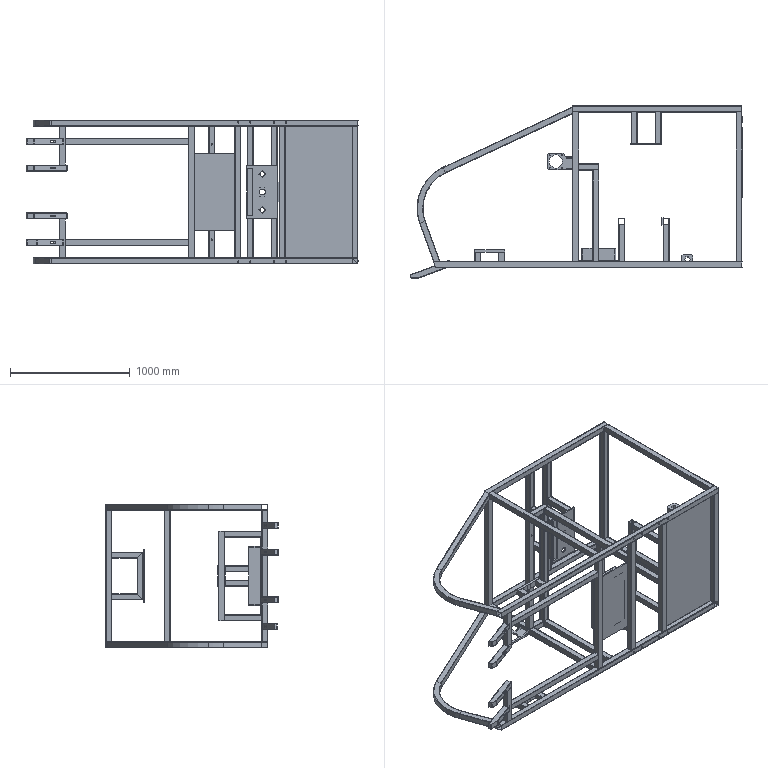Part | SolidWorks | features ICE 14, HoleWzd 6, Fillet 5, FlatPattern 4, CirPattern 3, Chamfer 2, Gusset 2, MirrorSolid 2, SMBaseFlange 2, SheetMetal 2, WeldCornerFeat 2, 3DProfileFeature 1, BossThin 1, LPattern 1, MirrorPattern 1, WeldMemberFeat 1, WeldmentFeature 1 | 71 solids | 1406 faces | box 2770 x 1437 x 1200 mm | volume 23055490 mm3 | plane 718 | cylinder 656 | torus 32 | commonest cylinder face diameters 3 x218 6 x212 11 x120 4.2 x24 8.5 x16 8 x12